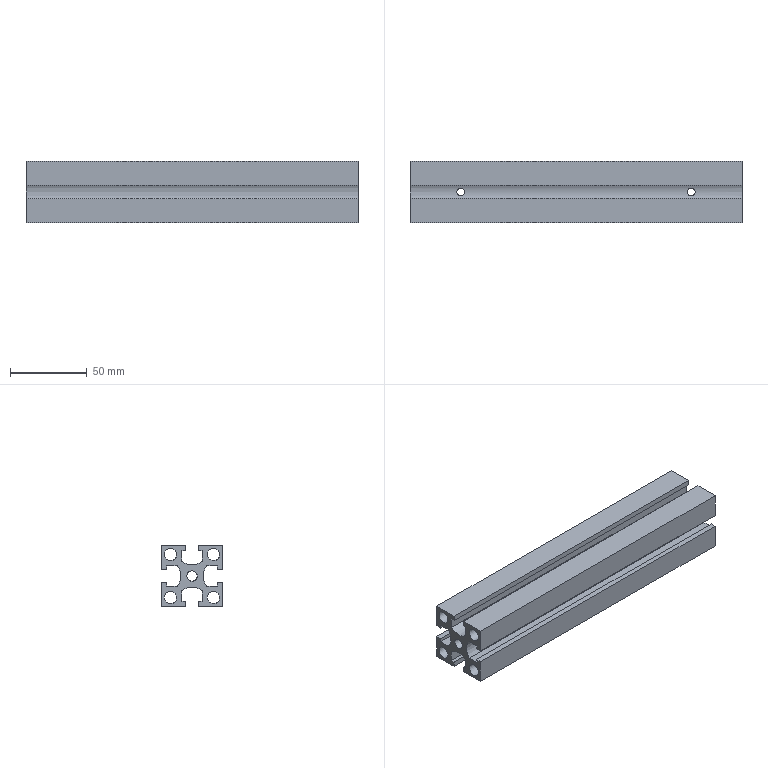Part | NX | 1 solid | 47 faces | box 216 x 40 x 40 mm | volume 171588 mm3 | plane 34 | cylinder 13 | commonest cylinder face diameters 5 x4 8 x4 20 x4 6.8 x1